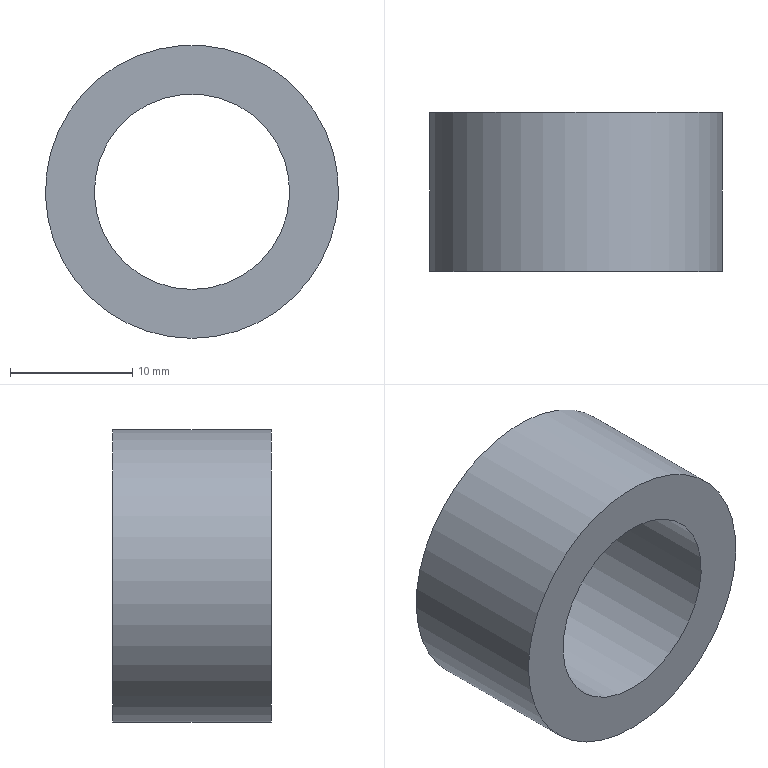Part | NX | features DATUM_CSYS 2, SKETCH 1, SWP104 1 | 1 solid | 4 faces | box 24 x 13 x 24 mm | volume 3267 mm3 | cylinder 2 | plane 2 | commonest cylinder face diameters 16 x1 24 x1
STEP:
#1=CARTESIAN_POINT('',(0.,-6.5,-8.));
#2=VERTEX_POINT('',#1);
#3=CARTESIAN_POINT('',(0.,-6.5,0.));
#4=DIRECTION('',(0.,-1.,0.));
#5=DIRECTION('',(0.,0.,-1.));
#6=AXIS2_PLACEMENT_3D('',#3,#4,#5);
#7=CIRCLE('',#6,8.);
#8=EDGE_CURVE('',#2,#2,#7,.T.);
#9=ORIENTED_EDGE('',*,*,#8,.T.);
#10=EDGE_LOOP('',(#9));
#11=FACE_BOUND('',#10,.T.);
#12=CARTESIAN_POINT('',(0.,6.5,-8.));
#13=VERTEX_POINT('',#12);
#14=CARTESIAN_POINT('',(0.,6.5,0.));
#15=DIRECTION('',(0.,-1.,0.));
#16=DIRECTION('',(0.,0.,-1.));
#17=AXIS2_PLACEMENT_3D('',#14,#15,#16);
#18=CIRCLE('',#17,8.);
#19=EDGE_CURVE('',#13,#13,#18,.T.);
#20=ORIENTED_EDGE('',*,*,#19,.F.);
#21=EDGE_LOOP('',(#20));
#22=FACE_BOUND('',#21,.T.);
#23=CARTESIAN_POINT('',(0.,0.,0.));
#24=DIRECTION('',(0.,-1.,0.));
#25=DIRECTION('',(0.,0.,-1.));
#26=AXIS2_PLACEMENT_3D('',#23,#24,#25);
#27=CYLINDRICAL_SURFACE('',#26,8.);
#28=ADVANCED_FACE('',(#11,#22),#27,.F.);
#29=CARTESIAN_POINT('',(0.,-6.5,-12.));
#30=VERTEX_POINT('',#29);
#31=CARTESIAN_POINT('',(0.,-6.5,0.));
#32=DIRECTION('',(0.,-1.,0.));
#33=DIRECTION('',(0.,0.,-1.));
#34=AXIS2_PLACEMENT_3D('',#31,#32,#33);
#35=CIRCLE('',#34,12.);
#36=EDGE_CURVE('',#30,#30,#35,.T.);
#37=ORIENTED_EDGE('',*,*,#36,.T.);
#38=EDGE_LOOP('',(#37));
#39=FACE_BOUND('',#38,.T.);
#40=ORIENTED_EDGE('',*,*,#8,.F.);
#41=EDGE_LOOP('',(#40));
#42=FACE_BOUND('',#41,.T.);
#43=CARTESIAN_POINT('',(8.,-6.5,0.));
#44=DIRECTION('',(0.,-1.,0.));
#45=DIRECTION('',(0.,0.,-1.));
#46=AXIS2_PLACEMENT_3D('',#43,#44,#45);
#47=PLANE('',#46);
#48=ADVANCED_FACE('',(#39,#42),#47,.T.);
#49=CARTESIAN_POINT('',(0.,6.5,-12.));
#50=VERTEX_POINT('',#49);
#51=CARTESIAN_POINT('',(0.,6.5,0.));
#52=DIRECTION('',(0.,-1.,0.));
#53=DIRECTION('',(0.,0.,-1.));
#54=AXIS2_PLACEMENT_3D('',#51,#52,#53);
#55=CIRCLE('',#54,12.);
#56=EDGE_CURVE('',#50,#50,#55,.T.);
#57=ORIENTED_EDGE('',*,*,#56,.T.);
#58=EDGE_LOOP('',(#57));
#59=FACE_BOUND('',#58,.T.);
#60=ORIENTED_EDGE('',*,*,#36,.F.);
#61=EDGE_LOOP('',(#60));
#62=FACE_BOUND('',#61,.T.);
#63=CARTESIAN_POINT('',(0.,0.,0.));
#64=DIRECTION('',(0.,-1.,0.));
#65=DIRECTION('',(0.,0.,-1.));
#66=AXIS2_PLACEMENT_3D('',#63,#64,#65);
#67=CYLINDRICAL_SURFACE('',#66,12.);
#68=ADVANCED_FACE('',(#59,#62),#67,.T.);
#69=ORIENTED_EDGE('',*,*,#19,.T.);
#70=EDGE_LOOP('',(#69));
#71=FACE_BOUND('',#70,.T.);
#72=ORIENTED_EDGE('',*,*,#56,.F.);
#73=EDGE_LOOP('',(#72));
#74=FACE_BOUND('',#73,.T.);
#75=CARTESIAN_POINT('',(12.,6.5,0.));
#76=DIRECTION('',(0.,1.,0.));
#77=DIRECTION('',(0.,0.,1.));
#78=AXIS2_PLACEMENT_3D('',#75,#76,#77);
#79=PLANE('',#78);
#80=ADVANCED_FACE('',(#71,#74),#79,.T.);
#81=CLOSED_SHELL('',(#28,#48,#68,#80));
#82=MANIFOLD_SOLID_BREP('',#81);
#83=(LENGTH_UNIT()NAMED_UNIT(*)SI_UNIT(.MILLI.,.METRE.));
#84=UNCERTAINTY_MEASURE_WITH_UNIT(LENGTH_MEASURE(0.00001),#83,'','');
#85=(NAMED_UNIT(*)PLANE_ANGLE_UNIT()SI_UNIT($,.RADIAN.));
#86=(NAMED_UNIT(*)SI_UNIT($,.STERADIAN.)SOLID_ANGLE_UNIT());
#87=(GEOMETRIC_REPRESENTATION_CONTEXT(3)GLOBAL_UNCERTAINTY_ASSIGNED_CONTEXT((#84))GLOBAL_UNIT_ASSIGNED_CONTEXT((#83,#85,#86))REPRESENTATION_CONTEXT('',''));
#88=ADVANCED_BREP_SHAPE_REPRESENTATION('',(#82),#87);